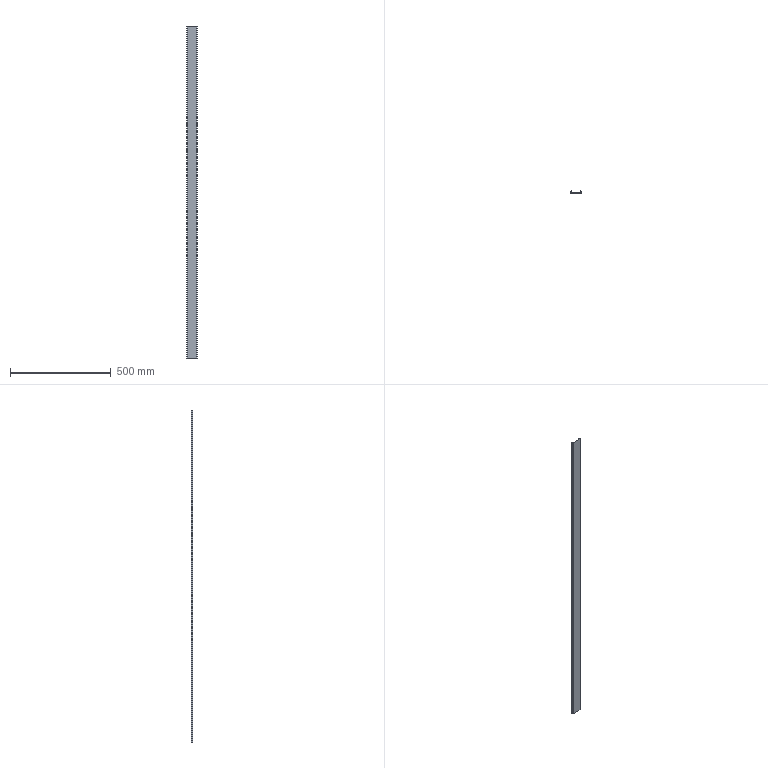Part | STEP file | 46A-00008CC12 | 1 solid | 32 faces | box 50 x 9.195 x 1650 mm | volume 144728 mm3 | plane 16 | cylinder 16 | commonest cylinder face diameters 1 x8 1.2 x6 2 x2
STEP:
#1=CARTESIAN_POINT('',(1.273,9.019,835.));
#2=VERTEX_POINT('',#1);
#3=CARTESIAN_POINT('',(0.4243,9.019,835.));
#4=VERTEX_POINT('',#3);
#5=CARTESIAN_POINT('',(1.273,9.019,835.));
#6=CARTESIAN_POINT('',(1.219,9.073,835.));
#7=CARTESIAN_POINT('',(1.158,9.118,835.));
#8=CARTESIAN_POINT('',(1.089,9.152,835.));
#9=CARTESIAN_POINT('',(0.9442,9.199,835.));
#10=CARTESIAN_POINT('',(0.7916,9.2,835.));
#11=CARTESIAN_POINT('',(0.7159,9.188,835.));
#12=CARTESIAN_POINT('',(0.6071,9.152,835.));
#13=CARTESIAN_POINT('',(0.5104,9.093,835.));
#14=CARTESIAN_POINT('',(0.4796,9.07,835.));
#15=CARTESIAN_POINT('',(0.4509,9.046,835.));
#16=CARTESIAN_POINT('',(0.4243,9.019,835.));
#17=B_SPLINE_CURVE_WITH_KNOTS('',5,(#5,#6,#7,#8,#9,#10,#11,#12,#13,#14,#15,#16),.UNSPECIFIED.,.F.,.U.,(6,3,3,6),(0.,0.5331,1.066,1.332),.UNSPECIFIED.);
#18=EDGE_CURVE('',#2,#4,#17,.T.);
#19=ORIENTED_EDGE('',*,*,#18,.T.);
#20=CARTESIAN_POINT('',(0.2485,8.595,835.));
#21=VERTEX_POINT('',#20);
#22=CARTESIAN_POINT('',(0.4243,9.019,835.));
#23=CARTESIAN_POINT('',(0.3843,8.979,835.));
#24=CARTESIAN_POINT('',(0.349,8.935,835.));
#25=CARTESIAN_POINT('',(0.3192,8.886,835.));
#26=CARTESIAN_POINT('',(0.2795,8.8,835.));
#27=CARTESIAN_POINT('',(0.2574,8.708,835.));
#28=CARTESIAN_POINT('',(0.2515,8.67,835.));
#29=CARTESIAN_POINT('',(0.2485,8.633,835.));
#30=CARTESIAN_POINT('',(0.2485,8.595,835.));
#31=B_SPLINE_CURVE_WITH_KNOTS('',5,(#22,#23,#24,#25,#26,#27,#28,#29,#30),.UNSPECIFIED.,.F.,.U.,(6,3,6),(0.,0.3999,0.6659),.UNSPECIFIED.);
#32=EDGE_CURVE('',#4,#21,#31,.T.);
#33=ORIENTED_EDGE('',*,*,#32,.T.);
#34=CARTESIAN_POINT('',(0.4243,8.171,835.));
#35=VERTEX_POINT('',#34);
#36=CARTESIAN_POINT('',(0.2485,8.595,835.));
#37=CARTESIAN_POINT('',(0.2485,8.538,835.));
#38=CARTESIAN_POINT('',(0.2552,8.482,835.));
#39=CARTESIAN_POINT('',(0.2685,8.426,835.));
#40=CARTESIAN_POINT('',(0.3014,8.337,835.));
#41=CARTESIAN_POINT('',(0.3507,8.257,835.));
#42=CARTESIAN_POINT('',(0.3731,8.226,835.));
#43=CARTESIAN_POINT('',(0.3977,8.197,835.));
#44=CARTESIAN_POINT('',(0.4243,8.171,835.));
#45=B_SPLINE_CURVE_WITH_KNOTS('',5,(#36,#37,#38,#39,#40,#41,#42,#43,#44),.UNSPECIFIED.,.F.,.U.,(6,3,6),(0.,0.3999,0.6659),.UNSPECIFIED.);
#46=EDGE_CURVE('',#21,#35,#45,.T.);
#47=ORIENTED_EDGE('',*,*,#46,.T.);
#48=CARTESIAN_POINT('',(2.898,5.697,835.));
#49=VERTEX_POINT('',#48);
#50=CARTESIAN_POINT('',(1.661,6.934,835.));
#51=DIRECTION('',(0.7071,-0.7071,0.));
#52=VECTOR('',#51,1.);
#53=LINE('',#50,#52);
#54=EDGE_CURVE('',#35,#49,#53,.T.);
#55=ORIENTED_EDGE('',*,*,#54,.T.);
#56=CARTESIAN_POINT('',(0.3706,5.02,835.));
#57=VERTEX_POINT('',#56);
#58=CARTESIAN_POINT('',(1.634,5.359,835.));
#59=DIRECTION('',(-0.9659,-0.2588,0.));
#60=VECTOR('',#59,1.);
#61=LINE('',#58,#60);
#62=EDGE_CURVE('',#49,#57,#61,.T.);
#63=ORIENTED_EDGE('',*,*,#62,.T.);
#64=CARTESIAN_POINT('',(0.,4.537,835.));
#65=VERTEX_POINT('',#64);
#66=CARTESIAN_POINT('',(0.3706,5.02,835.));
#67=CARTESIAN_POINT('',(0.32,5.007,835.));
#68=CARTESIAN_POINT('',(0.2712,4.986,835.));
#69=CARTESIAN_POINT('',(0.2253,4.96,835.));
#70=CARTESIAN_POINT('',(0.1416,4.896,835.));
#71=CARTESIAN_POINT('',(0.07725,4.812,835.));
#72=CARTESIAN_POINT('',(0.05076,4.766,835.));
#73=CARTESIAN_POINT('',(0.02052,4.693,835.));
#74=CARTESIAN_POINT('',(0.005155,4.616,835.));
#75=CARTESIAN_POINT('',(0.001709,4.589,835.));
#76=CARTESIAN_POINT('',(0.,4.563,835.));
#77=CARTESIAN_POINT('',(0.,4.537,835.));
#78=B_SPLINE_CURVE_WITH_KNOTS('',5,(#66,#67,#68,#69,#70,#71,#72,#73,#74,#75,#76,#77),.UNSPECIFIED.,.F.,.U.,(6,3,3,6),(0.,0.3702,0.7405,0.9253),.UNSPECIFIED.);
#79=EDGE_CURVE('',#57,#65,#78,.T.);
#80=ORIENTED_EDGE('',*,*,#79,.T.);
#81=CARTESIAN_POINT('',(0.,1.,835.));
#82=VERTEX_POINT('',#81);
#83=CARTESIAN_POINT('',(0.,2.769,835.));
#84=DIRECTION('',(0.,-1.,0.));
#85=VECTOR('',#84,1.);
#86=LINE('',#83,#85);
#87=EDGE_CURVE('',#65,#82,#86,.T.);
#88=ORIENTED_EDGE('',*,*,#87,.T.);
#89=CARTESIAN_POINT('',(1.,0.,835.));
#90=VERTEX_POINT('',#89);
#91=CARTESIAN_POINT('',(0.,1.,835.));
#92=CARTESIAN_POINT('',(0.,0.902,835.));
#93=CARTESIAN_POINT('',(0.012,0.804,835.));
#94=CARTESIAN_POINT('',(0.036,0.708,835.));
#95=CARTESIAN_POINT('',(0.107,0.5238,835.));
#96=CARTESIAN_POINT('',(0.2204,0.3622,835.));
#97=CARTESIAN_POINT('',(0.2868,0.2888,835.));
#98=CARTESIAN_POINT('',(0.4361,0.1597,835.));
#99=CARTESIAN_POINT('',(0.6122,0.0704,835.));
#100=CARTESIAN_POINT('',(0.7053,0.03682,835.));
#101=CARTESIAN_POINT('',(0.8215,0.01049,835.));
#102=CARTESIAN_POINT('',(0.9393,0.001534,835.));
#103=CARTESIAN_POINT('',(0.9596,0.0005109,835.));
#104=CARTESIAN_POINT('',(0.9798,0.000000001,835.));
#105=CARTESIAN_POINT('',(1.,0.000000001,835.));
#106=B_SPLINE_CURVE_WITH_KNOTS('',5,(#91,#92,#93,#94,#95,#96,#97,#98,#99,#100,#101,#102,#103,#104,#105),.UNSPECIFIED.,.F.,.U.,(6,3,3,3,6),(0.,0.6928,1.386,2.078,2.221),.UNSPECIFIED.);
#107=EDGE_CURVE('',#82,#90,#106,.T.);
#108=ORIENTED_EDGE('',*,*,#107,.T.);
#109=CARTESIAN_POINT('',(49.,0.,835.));
#110=VERTEX_POINT('',#109);
#111=CARTESIAN_POINT('',(25.,0.000000001,835.));
#112=DIRECTION('',(1.,0.,0.));
#113=VECTOR('',#112,1.);
#114=LINE('',#111,#113);
#115=EDGE_CURVE('',#90,#110,#114,.T.);
#116=ORIENTED_EDGE('',*,*,#115,.T.);
#117=CARTESIAN_POINT('',(50.,1.,835.));
#118=VERTEX_POINT('',#117);
#119=CARTESIAN_POINT('',(49.,0.000000001,835.));
#120=CARTESIAN_POINT('',(49.098,0.000000001,835.));
#121=CARTESIAN_POINT('',(49.196,0.012,835.));
#122=CARTESIAN_POINT('',(49.292,0.036,835.));
#123=CARTESIAN_POINT('',(49.476,0.107,835.));
#124=CARTESIAN_POINT('',(49.638,0.2204,835.));
#125=CARTESIAN_POINT('',(49.711,0.2868,835.));
#126=CARTESIAN_POINT('',(49.84,0.4361,835.));
#127=CARTESIAN_POINT('',(49.93,0.6122,835.));
#128=CARTESIAN_POINT('',(49.963,0.7053,835.));
#129=CARTESIAN_POINT('',(49.99,0.8215,835.));
#130=CARTESIAN_POINT('',(49.998,0.9393,835.));
#131=CARTESIAN_POINT('',(49.999,0.9596,835.));
#132=CARTESIAN_POINT('',(50.,0.9798,835.));
#133=CARTESIAN_POINT('',(50.,1.,835.));
#134=B_SPLINE_CURVE_WITH_KNOTS('',5,(#119,#120,#121,#122,#123,#124,#125,#126,#127,#128,#129,#130,#131,#132,#133),.UNSPECIFIED.,.F.,.U.,(6,3,3,3,6),(0.,0.6928,1.386,2.078,2.221),.UNSPECIFIED.);
#135=EDGE_CURVE('',#110,#118,#134,.T.);
#136=ORIENTED_EDGE('',*,*,#135,.T.);
#137=CARTESIAN_POINT('',(50.,4.537,835.));
#138=VERTEX_POINT('',#137);
#139=CARTESIAN_POINT('',(50.,2.769,835.));
#140=DIRECTION('',(0.,1.,0.));
#141=VECTOR('',#140,1.);
#142=LINE('',#139,#141);
#143=EDGE_CURVE('',#118,#138,#142,.T.);
#144=ORIENTED_EDGE('',*,*,#143,.T.);
#145=CARTESIAN_POINT('',(49.629,5.02,835.));
#146=VERTEX_POINT('',#145);
#147=CARTESIAN_POINT('',(50.,4.537,835.));
#148=CARTESIAN_POINT('',(50.,4.589,835.));
#149=CARTESIAN_POINT('',(49.993,4.642,835.));
#150=CARTESIAN_POINT('',(49.979,4.693,835.));
#151=CARTESIAN_POINT('',(49.939,4.791,835.));
#152=CARTESIAN_POINT('',(49.875,4.874,835.));
#153=CARTESIAN_POINT('',(49.837,4.912,835.));
#154=CARTESIAN_POINT('',(49.774,4.96,835.));
#155=CARTESIAN_POINT('',(49.704,4.995,835.));
#156=CARTESIAN_POINT('',(49.679,5.005,835.));
#157=CARTESIAN_POINT('',(49.655,5.013,835.));
#158=CARTESIAN_POINT('',(49.629,5.02,835.));
#159=B_SPLINE_CURVE_WITH_KNOTS('',5,(#147,#148,#149,#150,#151,#152,#153,#154,#155,#156,#157,#158),.UNSPECIFIED.,.F.,.U.,(6,3,3,6),(0.,0.3702,0.7405,0.9253),.UNSPECIFIED.);
#160=EDGE_CURVE('',#138,#146,#159,.T.);
#161=ORIENTED_EDGE('',*,*,#160,.T.);
#162=CARTESIAN_POINT('',(47.102,5.697,835.));
#163=VERTEX_POINT('',#162);
#164=CARTESIAN_POINT('',(48.366,5.359,835.));
#165=DIRECTION('',(-0.9659,0.2588,0.));
#166=VECTOR('',#165,1.);
#167=LINE('',#164,#166);
#168=EDGE_CURVE('',#146,#163,#167,.T.);
#169=ORIENTED_EDGE('',*,*,#168,.T.);
#170=CARTESIAN_POINT('',(49.576,8.171,835.));
#171=VERTEX_POINT('',#170);
#172=CARTESIAN_POINT('',(48.339,6.934,835.));
#173=DIRECTION('',(0.7071,0.7071,0.));
#174=VECTOR('',#173,1.);
#175=LINE('',#172,#174);
#176=EDGE_CURVE('',#163,#171,#175,.T.);
#177=ORIENTED_EDGE('',*,*,#176,.T.);
#178=CARTESIAN_POINT('',(49.751,8.595,835.));
#179=VERTEX_POINT('',#178);
#180=CARTESIAN_POINT('',(49.576,8.171,835.));
#181=CARTESIAN_POINT('',(49.629,8.224,835.));
#182=CARTESIAN_POINT('',(49.674,8.286,835.));
#183=CARTESIAN_POINT('',(49.709,8.354,835.));
#184=CARTESIAN_POINT('',(49.738,8.445,835.));
#185=CARTESIAN_POINT('',(49.749,8.539,835.));
#186=CARTESIAN_POINT('',(49.751,8.557,835.));
#187=CARTESIAN_POINT('',(49.751,8.576,835.));
#188=CARTESIAN_POINT('',(49.751,8.595,835.));
#189=B_SPLINE_CURVE_WITH_KNOTS('',5,(#180,#181,#182,#183,#184,#185,#186,#187,#188),.UNSPECIFIED.,.F.,.U.,(6,3,6),(0.,0.5331,0.6664),.UNSPECIFIED.);
#190=EDGE_CURVE('',#171,#179,#189,.T.);
#191=ORIENTED_EDGE('',*,*,#190,.T.);
#192=CARTESIAN_POINT('',(49.576,9.019,835.));
#193=VERTEX_POINT('',#192);
#194=CARTESIAN_POINT('',(49.751,8.595,835.));
#195=CARTESIAN_POINT('',(49.751,8.652,835.));
#196=CARTESIAN_POINT('',(49.745,8.708,835.));
#197=CARTESIAN_POINT('',(49.731,8.764,835.));
#198=CARTESIAN_POINT('',(49.699,8.853,835.));
#199=CARTESIAN_POINT('',(49.649,8.933,835.));
#200=CARTESIAN_POINT('',(49.627,8.964,835.));
#201=CARTESIAN_POINT('',(49.602,8.993,835.));
#202=CARTESIAN_POINT('',(49.576,9.019,835.));
#203=B_SPLINE_CURVE_WITH_KNOTS('',5,(#194,#195,#196,#197,#198,#199,#200,#201,#202),.UNSPECIFIED.,.F.,.U.,(6,3,6),(0.6664,1.066,1.332),.UNSPECIFIED.);
#204=EDGE_CURVE('',#179,#193,#203,.T.);
#205=ORIENTED_EDGE('',*,*,#204,.T.);
#206=CARTESIAN_POINT('',(48.727,9.019,835.));
#207=VERTEX_POINT('',#206);
#208=CARTESIAN_POINT('',(49.576,9.019,835.));
#209=CARTESIAN_POINT('',(49.522,9.073,835.));
#210=CARTESIAN_POINT('',(49.461,9.118,835.));
#211=CARTESIAN_POINT('',(49.392,9.152,835.));
#212=CARTESIAN_POINT('',(49.247,9.199,835.));
#213=CARTESIAN_POINT('',(49.095,9.2,835.));
#214=CARTESIAN_POINT('',(49.019,9.188,835.));
#215=CARTESIAN_POINT('',(48.91,9.152,835.));
#216=CARTESIAN_POINT('',(48.813,9.093,835.));
#217=CARTESIAN_POINT('',(48.782,9.07,835.));
#218=CARTESIAN_POINT('',(48.754,9.046,835.));
#219=CARTESIAN_POINT('',(48.727,9.019,835.));
#220=B_SPLINE_CURVE_WITH_KNOTS('',5,(#208,#209,#210,#211,#212,#213,#214,#215,#216,#217,#218,#219),.UNSPECIFIED.,.F.,.U.,(6,3,3,6),(0.,0.5331,1.066,1.332),.UNSPECIFIED.);
#221=EDGE_CURVE('',#193,#207,#220,.T.);
#222=ORIENTED_EDGE('',*,*,#221,.T.);
#223=CARTESIAN_POINT('',(45.396,5.688,835.));
#224=VERTEX_POINT('',#223);
#225=CARTESIAN_POINT('',(47.062,7.354,835.));
#226=DIRECTION('',(-0.7071,-0.7071,0.));
#227=VECTOR('',#226,1.);
#228=LINE('',#225,#227);
#229=EDGE_CURVE('',#207,#224,#228,.T.);
#230=ORIENTED_EDGE('',*,*,#229,.T.);
#231=CARTESIAN_POINT('',(45.25,5.335,835.));
#232=VERTEX_POINT('',#231);
#233=CARTESIAN_POINT('',(45.396,5.688,835.));
#234=CARTESIAN_POINT('',(45.363,5.655,835.));
#235=CARTESIAN_POINT('',(45.334,5.618,835.));
#236=CARTESIAN_POINT('',(45.309,5.577,835.));
#237=CARTESIAN_POINT('',(45.276,5.506,835.));
#238=CARTESIAN_POINT('',(45.257,5.429,835.));
#239=CARTESIAN_POINT('',(45.252,5.398,835.));
#240=CARTESIAN_POINT('',(45.25,5.366,835.));
#241=CARTESIAN_POINT('',(45.25,5.335,835.));
#242=B_SPLINE_CURVE_WITH_KNOTS('',5,(#233,#234,#235,#236,#237,#238,#239,#240,#241),.UNSPECIFIED.,.F.,.U.,(6,3,6),(0.,0.3332,0.5549),.UNSPECIFIED.);
#243=EDGE_CURVE('',#224,#232,#242,.T.);
#244=ORIENTED_EDGE('',*,*,#243,.T.);
#245=CARTESIAN_POINT('',(45.621,4.852,835.));
#246=VERTEX_POINT('',#245);
#247=CARTESIAN_POINT('',(45.25,5.335,835.));
#248=CARTESIAN_POINT('',(45.25,5.283,835.));
#249=CARTESIAN_POINT('',(45.257,5.23,835.));
#250=CARTESIAN_POINT('',(45.27,5.179,835.));
#251=CARTESIAN_POINT('',(45.311,5.081,835.));
#252=CARTESIAN_POINT('',(45.375,4.998,835.));
#253=CARTESIAN_POINT('',(45.413,4.96,835.));
#254=CARTESIAN_POINT('',(45.476,4.912,835.));
#255=CARTESIAN_POINT('',(45.546,4.877,835.));
#256=CARTESIAN_POINT('',(45.57,4.867,835.));
#257=CARTESIAN_POINT('',(45.595,4.859,835.));
#258=CARTESIAN_POINT('',(45.621,4.852,835.));
#259=B_SPLINE_CURVE_WITH_KNOTS('',5,(#247,#248,#249,#250,#251,#252,#253,#254,#255,#256,#257,#258),.UNSPECIFIED.,.F.,.U.,(6,3,3,6),(0.,0.3702,0.7405,0.9253),.UNSPECIFIED.);
#260=EDGE_CURVE('',#232,#246,#259,.T.);
#261=ORIENTED_EDGE('',*,*,#260,.T.);
#262=CARTESIAN_POINT('',(48.8,4.,835.));
#263=VERTEX_POINT('',#262);
#264=CARTESIAN_POINT('',(47.21,4.426,835.));
#265=DIRECTION('',(0.9659,-0.2588,0.));
#266=VECTOR('',#265,1.);
#267=LINE('',#264,#266);
#268=EDGE_CURVE('',#246,#263,#267,.T.);
#269=ORIENTED_EDGE('',*,*,#268,.T.);
#270=CARTESIAN_POINT('',(48.8,1.7,835.));
#271=VERTEX_POINT('',#270);
#272=CARTESIAN_POINT('',(48.8,2.85,835.));
#273=DIRECTION('',(0.,-1.,0.));
#274=VECTOR('',#273,1.);
#275=LINE('',#272,#274);
#276=EDGE_CURVE('',#263,#271,#275,.T.);
#277=ORIENTED_EDGE('',*,*,#276,.T.);
#278=CARTESIAN_POINT('',(48.3,1.2,835.));
#279=VERTEX_POINT('',#278);
#280=CARTESIAN_POINT('',(48.3,1.7,835.));
#281=DIRECTION('',(0.,0.,-1.));
#282=AXIS2_PLACEMENT_3D('',#280,#281,$);
#283=CIRCLE('',#282,0.5);
#284=EDGE_CURVE('',#271,#279,#283,.T.);
#285=ORIENTED_EDGE('',*,*,#284,.T.);
#286=CARTESIAN_POINT('',(1.7,1.2,835.));
#287=VERTEX_POINT('',#286);
#288=CARTESIAN_POINT('',(25.,1.2,835.));
#289=DIRECTION('',(-1.,0.,0.));
#290=VECTOR('',#289,1.);
#291=LINE('',#288,#290);
#292=EDGE_CURVE('',#279,#287,#291,.T.);
#293=ORIENTED_EDGE('',*,*,#292,.T.);
#294=CARTESIAN_POINT('',(1.2,1.7,835.));
#295=VERTEX_POINT('',#294);
#296=CARTESIAN_POINT('',(1.7,1.7,835.));
#297=DIRECTION('',(0.,0.,-1.));
#298=AXIS2_PLACEMENT_3D('',#296,#297,$);
#299=CIRCLE('',#298,0.5);
#300=EDGE_CURVE('',#287,#295,#299,.T.);
#301=ORIENTED_EDGE('',*,*,#300,.T.);
#302=CARTESIAN_POINT('',(1.2,4.,835.));
#303=VERTEX_POINT('',#302);
#304=CARTESIAN_POINT('',(1.2,2.85,835.));
#305=DIRECTION('',(0.,1.,0.));
#306=VECTOR('',#305,1.);
#307=LINE('',#304,#306);
#308=EDGE_CURVE('',#295,#303,#307,.T.);
#309=ORIENTED_EDGE('',*,*,#308,.T.);
#310=CARTESIAN_POINT('',(4.379,4.852,835.));
#311=VERTEX_POINT('',#310);
#312=CARTESIAN_POINT('',(2.79,4.426,835.));
#313=DIRECTION('',(0.9659,0.2588,0.));
#314=VECTOR('',#313,1.);
#315=LINE('',#312,#314);
#316=EDGE_CURVE('',#303,#311,#315,.T.);
#317=ORIENTED_EDGE('',*,*,#316,.T.);
#318=CARTESIAN_POINT('',(4.75,5.335,835.));
#319=VERTEX_POINT('',#318);
#320=CARTESIAN_POINT('',(4.379,4.852,835.));
#321=CARTESIAN_POINT('',(4.446,4.87,835.));
#322=CARTESIAN_POINT('',(4.51,4.899,835.));
#323=CARTESIAN_POINT('',(4.568,4.94,835.));
#324=CARTESIAN_POINT('',(4.662,5.034,835.));
#325=CARTESIAN_POINT('',(4.722,5.152,835.));
#326=CARTESIAN_POINT('',(4.741,5.212,835.));
#327=CARTESIAN_POINT('',(4.75,5.273,835.));
#328=CARTESIAN_POINT('',(4.75,5.335,835.));
#329=B_SPLINE_CURVE_WITH_KNOTS('',5,(#320,#321,#322,#323,#324,#325,#326,#327,#328),.UNSPECIFIED.,.F.,.U.,(6,3,6),(0.,0.4899,0.9256),.UNSPECIFIED.);
#330=EDGE_CURVE('',#311,#319,#329,.T.);
#331=ORIENTED_EDGE('',*,*,#330,.T.);
#332=CARTESIAN_POINT('',(4.604,5.688,835.));
#333=VERTEX_POINT('',#332);
#334=CARTESIAN_POINT('',(4.75,5.335,835.));
#335=CARTESIAN_POINT('',(4.75,5.343,835.));
#336=CARTESIAN_POINT('',(4.75,5.35,835.));
#337=CARTESIAN_POINT('',(4.75,5.358,835.));
#338=CARTESIAN_POINT('',(4.745,5.435,835.));
#339=CARTESIAN_POINT('',(4.726,5.51,835.));
#340=CARTESIAN_POINT('',(4.697,5.575,835.));
#341=CARTESIAN_POINT('',(4.657,5.634,835.));
#342=CARTESIAN_POINT('',(4.607,5.685,835.));
#343=CARTESIAN_POINT('',(4.606,5.686,835.));
#344=CARTESIAN_POINT('',(4.605,5.687,835.));
#345=CARTESIAN_POINT('',(4.604,5.688,835.));
#346=B_SPLINE_CURVE_WITH_KNOTS('',5,(#334,#335,#336,#337,#338,#339,#340,#341,#342,#343,#344,#345),.UNSPECIFIED.,.F.,.U.,(6,3,3,6),(0.9256,0.9798,1.47,1.481),.UNSPECIFIED.);
#347=EDGE_CURVE('',#319,#333,#346,.T.);
#348=ORIENTED_EDGE('',*,*,#347,.T.);
#349=CARTESIAN_POINT('',(2.938,7.354,835.));
#350=DIRECTION('',(-0.7071,0.7071,0.));
#351=VECTOR('',#350,1.);
#352=LINE('',#349,#351);
#353=EDGE_CURVE('',#333,#2,#352,.T.);
#354=ORIENTED_EDGE('',*,*,#353,.T.);
#355=EDGE_LOOP('',(#19,#33,#47,#55,#63,#80,#88,#108,#116,#136,#144,#161,#169,#177,#191,#205,#222,#230,#244,#261,#269,#277,#285,#293,#301,#309,#317,#331,#348,#354));
#356=FACE_OUTER_BOUND('',#355,.T.);
#357=CARTESIAN_POINT('',(0.,1.2,835.));
#358=DIRECTION('',(0.,0.,-1.));
#359=DIRECTION('',(-1.,0.,0.));
#360=AXIS2_PLACEMENT_3D('',#357,#358,#359);
#361=PLANE('',#360);
#362=ADVANCED_FACE('',(#356),#361,.F.);
#363=CARTESIAN_POINT('',(1.273,9.019,-815.));
#364=VERTEX_POINT('',#363);
#365=CARTESIAN_POINT('',(4.604,5.688,-815.));
#366=VERTEX_POINT('',#365);
#367=CARTESIAN_POINT('',(2.938,7.354,-815.));
#368=DIRECTION('',(0.7071,-0.7071,0.));
#369=VECTOR('',#368,1.);
#370=LINE('',#367,#369);
#371=EDGE_CURVE('',#364,#366,#370,.T.);
#372=ORIENTED_EDGE('',*,*,#371,.F.);
#373=CARTESIAN_POINT('',(1.273,9.019,10.));
#374=DIRECTION('',(0.,0.,1.));
#375=VECTOR('',#374,1.);
#376=LINE('',#373,#375);
#377=EDGE_CURVE('',#364,#2,#376,.T.);
#378=ORIENTED_EDGE('',*,*,#377,.T.);
#379=ORIENTED_EDGE('',*,*,#353,.F.);
#380=CARTESIAN_POINT('',(4.604,5.688,10.));
#381=DIRECTION('',(0.,0.,-1.));
#382=VECTOR('',#381,1.);
#383=LINE('',#380,#382);
#384=EDGE_CURVE('',#333,#366,#383,.T.);
#385=ORIENTED_EDGE('',*,*,#384,.T.);
#386=EDGE_LOOP('',(#372,#378,#379,#385));
#387=FACE_OUTER_BOUND('',#386,.T.);
#388=CARTESIAN_POINT('',(5.216,5.076,835.));
#389=DIRECTION('',(-0.7071,-0.7071,0.));
#390=DIRECTION('',(0.7071,-0.7071,0.));
#391=AXIS2_PLACEMENT_3D('',#388,#389,#390);
#392=PLANE('',#391);
#393=ADVANCED_FACE('',(#387),#392,.F.);
#394=ORIENTED_EDGE('',*,*,#384,.F.);
#395=ORIENTED_EDGE('',*,*,#347,.F.);
#396=CARTESIAN_POINT('',(4.75,5.335,-815.));
#397=VERTEX_POINT('',#396);
#398=CARTESIAN_POINT('',(4.75,5.335,835.));
#399=DIRECTION('',(0.,0.,-1.));
#400=VECTOR('',#399,1.);
#401=LINE('',#398,#400);
#402=EDGE_CURVE('',#319,#397,#401,.T.);
#403=ORIENTED_EDGE('',*,*,#402,.T.);
#404=CARTESIAN_POINT('',(4.25,5.335,-815.));
#405=DIRECTION('',(0.,0.,-1.));
#406=AXIS2_PLACEMENT_3D('',#404,#405,$);
#407=CIRCLE('',#406,0.5);
#408=EDGE_CURVE('',#366,#397,#407,.T.);
#409=ORIENTED_EDGE('',*,*,#408,.F.);
#410=EDGE_LOOP('',(#394,#395,#403,#409));
#411=FACE_OUTER_BOUND('',#410,.T.);
#412=CARTESIAN_POINT('',(4.25,5.335,835.));
#413=DIRECTION('',(0.,0.,-1.));
#414=DIRECTION('',(-1.,0.,0.));
#415=AXIS2_PLACEMENT_3D('',#412,#413,#414);
#416=CYLINDRICAL_SURFACE('',#415,0.5);
#417=ADVANCED_FACE('',(#411),#416,.T.);
#418=ORIENTED_EDGE('',*,*,#402,.F.);
#419=ORIENTED_EDGE('',*,*,#330,.F.);
#420=CARTESIAN_POINT('',(4.379,4.852,-815.));
#421=VERTEX_POINT('',#420);
#422=CARTESIAN_POINT('',(4.379,4.852,835.));
#423=DIRECTION('',(0.,0.,-1.));
#424=VECTOR('',#423,1.);
#425=LINE('',#422,#424);
#426=EDGE_CURVE('',#421,#311,#425,.F.);
#427=ORIENTED_EDGE('',*,*,#426,.F.);
#428=CARTESIAN_POINT('',(4.25,5.335,-815.));
#429=DIRECTION('',(0.,0.,-1.));
#430=AXIS2_PLACEMENT_3D('',#428,#429,$);
#431=CIRCLE('',#430,0.5);
#432=EDGE_CURVE('',#397,#421,#431,.T.);
#433=ORIENTED_EDGE('',*,*,#432,.F.);
#434=EDGE_LOOP('',(#418,#419,#427,#433));
#435=FACE_OUTER_BOUND('',#434,.T.);
#436=CARTESIAN_POINT('',(4.25,5.335,835.));
#437=DIRECTION('',(0.,0.,-1.));
#438=DIRECTION('',(1.,0.,0.));
#439=AXIS2_PLACEMENT_3D('',#436,#437,#438);
#440=CYLINDRICAL_SURFACE('',#439,0.5);
#441=ADVANCED_FACE('',(#435),#440,.T.);
#442=ORIENTED_EDGE('',*,*,#316,.F.);
#443=CARTESIAN_POINT('',(1.2,4.,-815.));
#444=VERTEX_POINT('',#443);
#445=CARTESIAN_POINT('',(1.2,4.,10.));
#446=DIRECTION('',(0.,0.,1.));
#447=VECTOR('',#446,1.);
#448=LINE('',#445,#447);
#449=EDGE_CURVE('',#444,#303,#448,.T.);
#450=ORIENTED_EDGE('',*,*,#449,.F.);
#451=CARTESIAN_POINT('',(2.79,4.426,-815.));
#452=DIRECTION('',(-0.9659,-0.2588,0.));
#453=VECTOR('',#452,1.);
#454=LINE('',#451,#453);
#455=EDGE_CURVE('',#421,#444,#454,.T.);
#456=ORIENTED_EDGE('',*,*,#455,.F.);
#457=ORIENTED_EDGE('',*,*,#426,.T.);
#458=EDGE_LOOP('',(#442,#450,#456,#457));
#459=FACE_OUTER_BOUND('',#458,.T.);
#460=CARTESIAN_POINT('',(1.2,4.,835.));
#461=DIRECTION('',(-0.2588,0.9659,0.));
#462=DIRECTION('',(-0.9659,-0.2588,0.));
#463=AXIS2_PLACEMENT_3D('',#460,#461,#462);
#464=PLANE('',#463);
#465=ADVANCED_FACE('',(#459),#464,.F.);
#466=ORIENTED_EDGE('',*,*,#308,.F.);
#467=CARTESIAN_POINT('',(1.2,1.7,-815.));
#468=VERTEX_POINT('',#467);
#469=CARTESIAN_POINT('',(1.2,1.7,10.));
#470=DIRECTION('',(0.,0.,-1.));
#471=VECTOR('',#470,1.);
#472=LINE('',#469,#471);
#473=EDGE_CURVE('',#295,#468,#472,.T.);
#474=ORIENTED_EDGE('',*,*,#473,.T.);
#475=CARTESIAN_POINT('',(1.2,2.85,-815.));
#476=DIRECTION('',(0.,-1.,0.));
#477=VECTOR('',#476,1.);
#478=LINE('',#475,#477);
#479=EDGE_CURVE('',#444,#468,#478,.T.);
#480=ORIENTED_EDGE('',*,*,#479,.F.);
#481=ORIENTED_EDGE('',*,*,#449,.T.);
#482=EDGE_LOOP('',(#466,#474,#480,#481));
#483=FACE_OUTER_BOUND('',#482,.T.);
#484=CARTESIAN_POINT('',(1.2,1.2,835.));
#485=DIRECTION('',(-1.,0.,0.));
#486=DIRECTION('',(0.,0.,1.));
#487=AXIS2_PLACEMENT_3D('',#484,#485,#486);
#488=PLANE('',#487);
#489=ADVANCED_FACE('',(#483),#488,.F.);
#490=ORIENTED_EDGE('',*,*,#300,.F.);
#491=CARTESIAN_POINT('',(1.7,1.2,-815.));
#492=VERTEX_POINT('',#491);
#493=CARTESIAN_POINT('',(1.7,1.2,835.));
#494=DIRECTION('',(0.,0.,1.));
#495=VECTOR('',#494,1.);
#496=LINE('',#493,#495);
#497=EDGE_CURVE('',#492,#287,#496,.T.);
#498=ORIENTED_EDGE('',*,*,#497,.F.);
#499=CARTESIAN_POINT('',(1.7,1.7,-815.));
#500=DIRECTION('',(0.,0.,1.));
#501=AXIS2_PLACEMENT_3D('',#499,#500,$);
#502=CIRCLE('',#501,0.5);
#503=EDGE_CURVE('',#468,#492,#502,.T.);
#504=ORIENTED_EDGE('',*,*,#503,.F.);
#505=ORIENTED_EDGE('',*,*,#473,.F.);
#506=EDGE_LOOP('',(#490,#498,#504,#505));
#507=FACE_OUTER_BOUND('',#506,.T.);
#508=CARTESIAN_POINT('',(1.7,1.7,835.));
#509=DIRECTION('',(0.,0.,1.));
#510=DIRECTION('',(-1.,0.,0.));
#511=AXIS2_PLACEMENT_3D('',#508,#509,#510);
#512=CYLINDRICAL_SURFACE('',#511,0.5);
#513=ADVANCED_FACE('',(#507),#512,.F.);
#514=ORIENTED_EDGE('',*,*,#292,.F.);
#515=CARTESIAN_POINT('',(48.3,1.2,-815.));
#516=VERTEX_POINT('',#515);
#517=CARTESIAN_POINT('',(48.3,1.2,10.));
#518=DIRECTION('',(0.,0.,-1.));
#519=VECTOR('',#518,1.);
#520=LINE('',#517,#519);
#521=EDGE_CURVE('',#279,#516,#520,.T.);
#522=ORIENTED_EDGE('',*,*,#521,.T.);
#523=CARTESIAN_POINT('',(25.,1.2,-815.));
#524=DIRECTION('',(1.,0.,0.));
#525=VECTOR('',#524,1.);
#526=LINE('',#523,#525);
#527=EDGE_CURVE('',#492,#516,#526,.T.);
#528=ORIENTED_EDGE('',*,*,#527,.F.);
#529=ORIENTED_EDGE('',*,*,#497,.T.);
#530=EDGE_LOOP('',(#514,#522,#528,#529));
#531=FACE_OUTER_BOUND('',#530,.T.);
#532=CARTESIAN_POINT('',(1.2,1.2,835.));
#533=DIRECTION('',(0.,-1.,0.));
#534=DIRECTION('',(0.,0.,-1.));
#535=AXIS2_PLACEMENT_3D('',#532,#533,#534);
#536=PLANE('',#535);
#537=ADVANCED_FACE('',(#531),#536,.F.);
#538=ORIENTED_EDGE('',*,*,#284,.F.);
#539=CARTESIAN_POINT('',(48.8,1.7,-815.));
#540=VERTEX_POINT('',#539);
#541=CARTESIAN_POINT('',(48.8,1.7,835.));
#542=DIRECTION('',(0.,0.,1.));
#543=VECTOR('',#542,1.);
#544=LINE('',#541,#543);
#545=EDGE_CURVE('',#540,#271,#544,.T.);
#546=ORIENTED_EDGE('',*,*,#545,.F.);
#547=CARTESIAN_POINT('',(48.3,1.7,-815.));
#548=DIRECTION('',(0.,0.,1.));
#549=AXIS2_PLACEMENT_3D('',#547,#548,$);
#550=CIRCLE('',#549,0.5);
#551=EDGE_CURVE('',#516,#540,#550,.T.);
#552=ORIENTED_EDGE('',*,*,#551,.F.);
#553=ORIENTED_EDGE('',*,*,#521,.F.);
#554=EDGE_LOOP('',(#538,#546,#552,#553));
#555=FACE_OUTER_BOUND('',#554,.T.);
#556=CARTESIAN_POINT('',(48.3,1.7,835.));
#557=DIRECTION('',(0.,0.,1.));
#558=DIRECTION('',(-1.,0.,0.));
#559=AXIS2_PLACEMENT_3D('',#556,#557,#558);
#560=CYLINDRICAL_SURFACE('',#559,0.5);
#561=ADVANCED_FACE('',(#555),#560,.F.);
#562=ORIENTED_EDGE('',*,*,#276,.F.);
#563=CARTESIAN_POINT('',(48.8,4.,-815.));
#564=VERTEX_POINT('',#563);
#565=CARTESIAN_POINT('',(48.8,4.,10.));
#566=DIRECTION('',(0.,0.,1.));
#567=VECTOR('',#566,1.);
#568=LINE('',#565,#567);
#569=EDGE_CURVE('',#564,#263,#568,.T.);
#570=ORIENTED_EDGE('',*,*,#569,.F.);
#571=CARTESIAN_POINT('',(48.8,2.85,-815.));
#572=DIRECTION('',(0.,1.,0.));
#573=VECTOR('',#572,1.);
#574=LINE('',#571,#573);
#575=EDGE_CURVE('',#540,#564,#574,.T.);
#576=ORIENTED_EDGE('',*,*,#575,.F.);
#577=ORIENTED_EDGE('',*,*,#545,.T.);
#578=EDGE_LOOP('',(#562,#570,#576,#577));
#579=FACE_OUTER_BOUND('',#578,.T.);
#580=CARTESIAN_POINT('',(48.8,1.2,835.));
#581=DIRECTION('',(1.,0.,0.));
#582=DIRECTION('',(0.,1.,0.));
#583=AXIS2_PLACEMENT_3D('',#580,#581,#582);
#584=PLANE('',#583);
#585=ADVANCED_FACE('',(#579),#584,.F.);
#586=ORIENTED_EDGE('',*,*,#268,.F.);
#587=CARTESIAN_POINT('',(45.621,4.852,-815.));
#588=VERTEX_POINT('',#587);
#589=CARTESIAN_POINT('',(45.621,4.852,10.));
#590=DIRECTION('',(0.,0.,-1.));
#591=VECTOR('',#590,1.);
#592=LINE('',#589,#591);
#593=EDGE_CURVE('',#246,#588,#592,.T.);
#594=ORIENTED_EDGE('',*,*,#593,.T.);
#595=CARTESIAN_POINT('',(47.21,4.426,-815.));
#596=DIRECTION('',(-0.9659,0.2588,0.));
#597=VECTOR('',#596,1.);
#598=LINE('',#595,#597);
#599=EDGE_CURVE('',#564,#588,#598,.T.);
#600=ORIENTED_EDGE('',*,*,#599,.F.);
#601=ORIENTED_EDGE('',*,*,#569,.T.);
#602=EDGE_LOOP('',(#586,#594,#600,#601));
#603=FACE_OUTER_BOUND('',#602,.T.);
#604=CARTESIAN_POINT('',(48.8,4.,835.));
#605=DIRECTION('',(0.2588,0.9659,0.));
#606=DIRECTION('',(-0.9659,0.2588,0.));
#607=AXIS2_PLACEMENT_3D('',#604,#605,#606);
#608=PLANE('',#607);
#609=ADVANCED_FACE('',(#603),#608,.F.);
#610=ORIENTED_EDGE('',*,*,#593,.F.);
#611=ORIENTED_EDGE('',*,*,#260,.F.);
#612=CARTESIAN_POINT('',(45.25,5.335,-815.));
#613=VERTEX_POINT('',#612);
#614=CARTESIAN_POINT('',(45.25,5.335,835.));
#615=DIRECTION('',(0.,0.,-1.));
#616=VECTOR('',#615,1.);
#617=LINE('',#614,#616);
#618=EDGE_CURVE('',#232,#613,#617,.T.);
#619=ORIENTED_EDGE('',*,*,#618,.T.);
#620=CARTESIAN_POINT('',(45.75,5.335,-815.));
#621=DIRECTION('',(0.,0.,-1.));
#622=AXIS2_PLACEMENT_3D('',#620,#621,$);
#623=CIRCLE('',#622,0.5);
#624=EDGE_CURVE('',#588,#613,#623,.T.);
#625=ORIENTED_EDGE('',*,*,#624,.F.);
#626=EDGE_LOOP('',(#610,#611,#619,#625));
#627=FACE_OUTER_BOUND('',#626,.T.);
#628=CARTESIAN_POINT('',(45.75,5.335,835.));
#629=DIRECTION('',(0.,0.,-1.));
#630=DIRECTION('',(1.,0.,0.));
#631=AXIS2_PLACEMENT_3D('',#628,#629,#630);
#632=CYLINDRICAL_SURFACE('',#631,0.5);
#633=ADVANCED_FACE('',(#627),#632,.T.);
#634=ORIENTED_EDGE('',*,*,#618,.F.);
#635=ORIENTED_EDGE('',*,*,#243,.F.);
#636=CARTESIAN_POINT('',(45.396,5.688,-815.));
#637=VERTEX_POINT('',#636);
#638=CARTESIAN_POINT('',(45.396,5.688,835.));
#639=DIRECTION('',(0.,0.,-1.));
#640=VECTOR('',#639,1.);
#641=LINE('',#638,#640);
#642=EDGE_CURVE('',#637,#224,#641,.F.);
#643=ORIENTED_EDGE('',*,*,#642,.F.);
#644=CARTESIAN_POINT('',(45.75,5.335,-815.));
#645=DIRECTION('',(0.,0.,-1.));
#646=AXIS2_PLACEMENT_3D('',#644,#645,$);
#647=CIRCLE('',#646,0.5);
#648=EDGE_CURVE('',#613,#637,#647,.T.);
#649=ORIENTED_EDGE('',*,*,#648,.F.);
#650=EDGE_LOOP('',(#634,#635,#643,#649));
#651=FACE_OUTER_BOUND('',#650,.T.);
#652=CARTESIAN_POINT('',(45.75,5.335,835.));
#653=DIRECTION('',(0.,0.,-1.));
#654=DIRECTION('',(-1.,0.,0.));
#655=AXIS2_PLACEMENT_3D('',#652,#653,#654);
#656=CYLINDRICAL_SURFACE('',#655,0.5);
#657=ADVANCED_FACE('',(#651),#656,.T.);
#658=ORIENTED_EDGE('',*,*,#229,.F.);
#659=CARTESIAN_POINT('',(48.727,9.019,-815.));
#660=VERTEX_POINT('',#659);
#661=CARTESIAN_POINT('',(48.727,9.019,10.));
#662=DIRECTION('',(0.,0.,-1.));
#663=VECTOR('',#662,1.);
#664=LINE('',#661,#663);
#665=EDGE_CURVE('',#207,#660,#664,.T.);
#666=ORIENTED_EDGE('',*,*,#665,.T.);
#667=CARTESIAN_POINT('',(47.062,7.354,-815.));
#668=DIRECTION('',(0.7071,0.7071,0.));
#669=VECTOR('',#668,1.);
#670=LINE('',#667,#669);
#671=EDGE_CURVE('',#637,#660,#670,.T.);
#672=ORIENTED_EDGE('',*,*,#671,.F.);
#673=ORIENTED_EDGE('',*,*,#642,.T.);
#674=EDGE_LOOP('',(#658,#666,#672,#673));
#675=FACE_OUTER_BOUND('',#674,.T.);
#676=CARTESIAN_POINT('',(44.784,5.076,835.));
#677=DIRECTION('',(0.7071,-0.7071,0.));
#678=DIRECTION('',(0.7071,0.7071,0.));
#679=AXIS2_PLACEMENT_3D('',#676,#677,#678);
#680=PLANE('',#679);
#681=ADVANCED_FACE('',(#675),#680,.F.);
#682=ORIENTED_EDGE('',*,*,#665,.F.);
#683=ORIENTED_EDGE('',*,*,#221,.F.);
#684=CARTESIAN_POINT('',(49.576,9.019,-815.));
#685=VERTEX_POINT('',#684);
#686=CARTESIAN_POINT('',(49.576,9.019,835.));
#687=DIRECTION('',(0.,0.,-1.));
#688=VECTOR('',#687,1.);
#689=LINE('',#686,#688);
#690=EDGE_CURVE('',#193,#685,#689,.T.);
#691=ORIENTED_EDGE('',*,*,#690,.T.);
#692=CARTESIAN_POINT('',(49.151,8.595,-815.));
#693=DIRECTION('',(0.,0.,-1.));
#694=AXIS2_PLACEMENT_3D('',#692,#693,$);
#695=CIRCLE('',#694,0.6);
#696=EDGE_CURVE('',#660,#685,#695,.T.);
#697=ORIENTED_EDGE('',*,*,#696,.F.);
#698=EDGE_LOOP('',(#682,#683,#691,#697));
#699=FACE_OUTER_BOUND('',#698,.T.);
#700=CARTESIAN_POINT('',(49.151,8.595,835.));
#701=DIRECTION('',(0.,0.,-1.));
#702=DIRECTION('',(-1.,0.,0.));
#703=AXIS2_PLACEMENT_3D('',#700,#701,#702);
#704=CYLINDRICAL_SURFACE('',#703,0.6);
#705=ADVANCED_FACE('',(#699),#704,.T.);
#706=ORIENTED_EDGE('',*,*,#690,.F.);
#707=ORIENTED_EDGE('',*,*,#204,.F.);
#708=CARTESIAN_POINT('',(49.751,8.595,-815.));
#709=VERTEX_POINT('',#708);
#710=CARTESIAN_POINT('',(49.751,8.595,835.));
#711=DIRECTION('',(0.,0.,-1.));
#712=VECTOR('',#711,1.);
#713=LINE('',#710,#712);
#714=EDGE_CURVE('',#179,#709,#713,.T.);
#715=ORIENTED_EDGE('',*,*,#714,.T.);
#716=CARTESIAN_POINT('',(49.151,8.595,-815.));
#717=DIRECTION('',(0.,0.,-1.));
#718=AXIS2_PLACEMENT_3D('',#716,#717,$);
#719=CIRCLE('',#718,0.6);
#720=EDGE_CURVE('',#685,#709,#719,.T.);
#721=ORIENTED_EDGE('',*,*,#720,.F.);
#722=EDGE_LOOP('',(#706,#707,#715,#721));
#723=FACE_OUTER_BOUND('',#722,.T.);
#724=CARTESIAN_POINT('',(49.151,8.595,835.));
#725=DIRECTION('',(0.,0.,-1.));
#726=DIRECTION('',(-1.,0.,0.));
#727=AXIS2_PLACEMENT_3D('',#724,#725,#726);
#728=CYLINDRICAL_SURFACE('',#727,0.6);
#729=ADVANCED_FACE('',(#723),#728,.T.);
#730=ORIENTED_EDGE('',*,*,#714,.F.);
#731=ORIENTED_EDGE('',*,*,#190,.F.);
#732=CARTESIAN_POINT('',(49.576,8.171,-815.));
#733=VERTEX_POINT('',#732);
#734=CARTESIAN_POINT('',(49.576,8.171,835.));
#735=DIRECTION('',(0.,0.,-1.));
#736=VECTOR('',#735,1.);
#737=LINE('',#734,#736);
#738=EDGE_CURVE('',#733,#171,#737,.F.);
#739=ORIENTED_EDGE('',*,*,#738,.F.);
#740=CARTESIAN_POINT('',(49.151,8.595,-815.));
#741=DIRECTION('',(0.,0.,-1.));
#742=AXIS2_PLACEMENT_3D('',#740,#741,$);
#743=CIRCLE('',#742,0.6);
#744=EDGE_CURVE('',#709,#733,#743,.T.);
#745=ORIENTED_EDGE('',*,*,#744,.F.);
#746=EDGE_LOOP('',(#730,#731,#739,#745));
#747=FACE_OUTER_BOUND('',#746,.T.);
#748=CARTESIAN_POINT('',(49.151,8.595,835.));
#749=DIRECTION('',(0.,0.,-1.));
#750=DIRECTION('',(1.,0.,0.));
#751=AXIS2_PLACEMENT_3D('',#748,#749,#750);
#752=CYLINDRICAL_SURFACE('',#751,0.6);
#753=ADVANCED_FACE('',(#747),#752,.T.);
#754=ORIENTED_EDGE('',*,*,#176,.F.);
#755=CARTESIAN_POINT('',(47.102,5.697,-815.));
#756=VERTEX_POINT('',#755);
#757=CARTESIAN_POINT('',(47.102,5.697,10.));
#758=DIRECTION('',(0.,0.,1.));
#759=VECTOR('',#758,1.);
#760=LINE('',#757,#759);
#761=EDGE_CURVE('',#756,#163,#760,.T.);
#762=ORIENTED_EDGE('',*,*,#761,.F.);
#763=CARTESIAN_POINT('',(48.339,6.934,-815.));
#764=DIRECTION('',(-0.7071,-0.7071,0.));
#765=VECTOR('',#764,1.);
#766=LINE('',#763,#765);
#767=EDGE_CURVE('',#733,#756,#766,.T.);
#768=ORIENTED_EDGE('',*,*,#767,.F.);
#769=ORIENTED_EDGE('',*,*,#738,.T.);
#770=EDGE_LOOP('',(#754,#762,#768,#769));
#771=FACE_OUTER_BOUND('',#770,.T.);
#772=CARTESIAN_POINT('',(47.102,5.697,835.));
#773=DIRECTION('',(-0.7071,0.7071,0.));
#774=DIRECTION('',(-0.7071,-0.7071,0.));
#775=AXIS2_PLACEMENT_3D('',#772,#773,#774);
#776=PLANE('',#775);
#777=ADVANCED_FACE('',(#771),#776,.F.);
#778=ORIENTED_EDGE('',*,*,#168,.F.);
#779=CARTESIAN_POINT('',(49.629,5.02,-815.));
#780=VERTEX_POINT('',#779);
#781=CARTESIAN_POINT('',(49.629,5.02,10.));
#782=DIRECTION('',(0.,0.,-1.));
#783=VECTOR('',#782,1.);
#784=LINE('',#781,#783);
#785=EDGE_CURVE('',#146,#780,#784,.T.);
#786=ORIENTED_EDGE('',*,*,#785,.T.);
#787=CARTESIAN_POINT('',(48.366,5.359,-815.));
#788=DIRECTION('',(0.9659,-0.2588,0.));
#789=VECTOR('',#788,1.);
#790=LINE('',#787,#789);
#791=EDGE_CURVE('',#756,#780,#790,.T.);
#792=ORIENTED_EDGE('',*,*,#791,.F.);
#793=ORIENTED_EDGE('',*,*,#761,.T.);
#794=EDGE_LOOP('',(#778,#786,#792,#793));
#795=FACE_OUTER_BOUND('',#794,.T.);
#796=CARTESIAN_POINT('',(50.,4.921,835.));
#797=DIRECTION('',(-0.2588,-0.9659,0.));
#798=DIRECTION('',(0.9659,-0.2588,0.));
#799=AXIS2_PLACEMENT_3D('',#796,#797,#798);
#800=PLANE('',#799);
#801=ADVANCED_FACE('',(#795),#800,.F.);
#802=ORIENTED_EDGE('',*,*,#785,.F.);
#803=ORIENTED_EDGE('',*,*,#160,.F.);
#804=CARTESIAN_POINT('',(50.,4.537,-815.));
#805=VERTEX_POINT('',#804);
#806=CARTESIAN_POINT('',(50.,4.537,835.));
#807=DIRECTION('',(0.,0.,-1.));
#808=VECTOR('',#807,1.);
#809=LINE('',#806,#808);
#810=EDGE_CURVE('',#805,#138,#809,.F.);
#811=ORIENTED_EDGE('',*,*,#810,.F.);
#812=CARTESIAN_POINT('',(49.5,4.537,-815.));
#813=DIRECTION('',(0.,0.,-1.));
#814=AXIS2_PLACEMENT_3D('',#812,#813,$);
#815=CIRCLE('',#814,0.5);
#816=EDGE_CURVE('',#780,#805,#815,.T.);
#817=ORIENTED_EDGE('',*,*,#816,.F.);
#818=EDGE_LOOP('',(#802,#803,#811,#817));
#819=FACE_OUTER_BOUND('',#818,.T.);
#820=CARTESIAN_POINT('',(49.5,4.537,835.));
#821=DIRECTION('',(0.,0.,-1.));
#822=DIRECTION('',(-1.,0.,0.));
#823=AXIS2_PLACEMENT_3D('',#820,#821,#822);
#824=CYLINDRICAL_SURFACE('',#823,0.5);
#825=ADVANCED_FACE('',(#819),#824,.T.);
#826=ORIENTED_EDGE('',*,*,#143,.F.);
#827=CARTESIAN_POINT('',(50.,1.,-815.));
#828=VERTEX_POINT('',#827);
#829=CARTESIAN_POINT('',(50.,1.,10.));
#830=DIRECTION('',(0.,0.,-1.));
#831=VECTOR('',#830,1.);
#832=LINE('',#829,#831);
#833=EDGE_CURVE('',#118,#828,#832,.T.);
#834=ORIENTED_EDGE('',*,*,#833,.T.);
#835=CARTESIAN_POINT('',(50.,2.769,-815.));
#836=DIRECTION('',(0.,-1.,0.));
#837=VECTOR('',#836,1.);
#838=LINE('',#835,#837);
#839=EDGE_CURVE('',#805,#828,#838,.T.);
#840=ORIENTED_EDGE('',*,*,#839,.F.);
#841=ORIENTED_EDGE('',*,*,#810,.T.);
#842=EDGE_LOOP('',(#826,#834,#840,#841));
#843=FACE_OUTER_BOUND('',#842,.T.);
#844=CARTESIAN_POINT('',(50.,0.,835.));
#845=DIRECTION('',(-1.,0.,0.));
#846=DIRECTION('',(0.,-1.,0.));
#847=AXIS2_PLACEMENT_3D('',#844,#845,#846);
#848=PLANE('',#847);
#849=ADVANCED_FACE('',(#843),#848,.F.);
#850=ORIENTED_EDGE('',*,*,#833,.F.);
#851=ORIENTED_EDGE('',*,*,#135,.F.);
#852=CARTESIAN_POINT('',(49.,0.,-815.));
#853=VERTEX_POINT('',#852);
#854=CARTESIAN_POINT('',(49.,0.,835.));
#855=DIRECTION('',(0.,0.,-1.));
#856=VECTOR('',#855,1.);
#857=LINE('',#854,#856);
#858=EDGE_CURVE('',#853,#110,#857,.F.);
#859=ORIENTED_EDGE('',*,*,#858,.F.);
#860=CARTESIAN_POINT('',(49.,1.,-815.));
#861=DIRECTION('',(0.,0.,-1.));
#862=AXIS2_PLACEMENT_3D('',#860,#861,$);
#863=CIRCLE('',#862,1.);
#864=EDGE_CURVE('',#828,#853,#863,.T.);
#865=ORIENTED_EDGE('',*,*,#864,.F.);
#866=EDGE_LOOP('',(#850,#851,#859,#865));
#867=FACE_OUTER_BOUND('',#866,.T.);
#868=CARTESIAN_POINT('',(49.,1.,835.));
#869=DIRECTION('',(0.,0.,-1.));
#870=DIRECTION('',(1.,0.,0.));
#871=AXIS2_PLACEMENT_3D('',#868,#869,#870);
#872=CYLINDRICAL_SURFACE('',#871,1.);
#873=ADVANCED_FACE('',(#867),#872,.T.);
#874=ORIENTED_EDGE('',*,*,#115,.F.);
#875=CARTESIAN_POINT('',(1.,0.,-815.));
#876=VERTEX_POINT('',#875);
#877=CARTESIAN_POINT('',(1.,0.,10.));
#878=DIRECTION('',(0.,0.,-1.));
#879=VECTOR('',#878,1.);
#880=LINE('',#877,#879);
#881=EDGE_CURVE('',#90,#876,#880,.T.);
#882=ORIENTED_EDGE('',*,*,#881,.T.);
#883=CARTESIAN_POINT('',(25.,0.,-815.));
#884=DIRECTION('',(-1.,0.,0.));
#885=VECTOR('',#884,1.);
#886=LINE('',#883,#885);
#887=EDGE_CURVE('',#853,#876,#886,.T.);
#888=ORIENTED_EDGE('',*,*,#887,.F.);
#889=ORIENTED_EDGE('',*,*,#858,.T.);
#890=EDGE_LOOP('',(#874,#882,#888,#889));
#891=FACE_OUTER_BOUND('',#890,.T.);
#892=CARTESIAN_POINT('',(0.,0.,835.));
#893=DIRECTION('',(0.,1.,0.));
#894=DIRECTION('',(-1.,0.,0.));
#895=AXIS2_PLACEMENT_3D('',#892,#893,#894);
#896=PLANE('',#895);
#897=ADVANCED_FACE('',(#891),#896,.F.);
#898=ORIENTED_EDGE('',*,*,#881,.F.);
#899=ORIENTED_EDGE('',*,*,#107,.F.);
#900=CARTESIAN_POINT('',(0.,1.,-815.));
#901=VERTEX_POINT('',#900);
#902=CARTESIAN_POINT('',(0.,1.,835.));
#903=DIRECTION('',(0.,0.,-1.));
#904=VECTOR('',#903,1.);
#905=LINE('',#902,#904);
#906=EDGE_CURVE('',#901,#82,#905,.F.);
#907=ORIENTED_EDGE('',*,*,#906,.F.);
#908=CARTESIAN_POINT('',(1.,1.,-815.));
#909=DIRECTION('',(0.,0.,-1.));
#910=AXIS2_PLACEMENT_3D('',#908,#909,$);
#911=CIRCLE('',#910,1.);
#912=EDGE_CURVE('',#876,#901,#911,.T.);
#913=ORIENTED_EDGE('',*,*,#912,.F.);
#914=EDGE_LOOP('',(#898,#899,#907,#913));
#915=FACE_OUTER_BOUND('',#914,.T.);
#916=CARTESIAN_POINT('',(1.,1.,835.));
#917=DIRECTION('',(0.,0.,-1.));
#918=DIRECTION('',(1.,0.,0.));
#919=AXIS2_PLACEMENT_3D('',#916,#917,#918);
#920=CYLINDRICAL_SURFACE('',#919,1.);
#921=ADVANCED_FACE('',(#915),#920,.T.);
#922=ORIENTED_EDGE('',*,*,#87,.F.);
#923=CARTESIAN_POINT('',(0.,4.537,-815.));
#924=VERTEX_POINT('',#923);
#925=CARTESIAN_POINT('',(0.,4.537,10.));
#926=DIRECTION('',(0.,0.,-1.));
#927=VECTOR('',#926,1.);
#928=LINE('',#925,#927);
#929=EDGE_CURVE('',#65,#924,#928,.T.);
#930=ORIENTED_EDGE('',*,*,#929,.T.);
#931=CARTESIAN_POINT('',(0.,2.769,-815.));
#932=DIRECTION('',(0.,1.,0.));
#933=VECTOR('',#932,1.);
#934=LINE('',#931,#933);
#935=EDGE_CURVE('',#901,#924,#934,.T.);
#936=ORIENTED_EDGE('',*,*,#935,.F.);
#937=ORIENTED_EDGE('',*,*,#906,.T.);
#938=EDGE_LOOP('',(#922,#930,#936,#937));
#939=FACE_OUTER_BOUND('',#938,.T.);
#940=CARTESIAN_POINT('',(0.,0.,835.));
#941=DIRECTION('',(1.,0.,0.));
#942=DIRECTION('',(0.,1.,0.));
#943=AXIS2_PLACEMENT_3D('',#940,#941,#942);
#944=PLANE('',#943);
#945=ADVANCED_FACE('',(#939),#944,.F.);
#946=ORIENTED_EDGE('',*,*,#929,.F.);
#947=ORIENTED_EDGE('',*,*,#79,.F.);
#948=CARTESIAN_POINT('',(0.3706,5.02,-815.));
#949=VERTEX_POINT('',#948);
#950=CARTESIAN_POINT('',(0.3706,5.02,835.));
#951=DIRECTION('',(0.,0.,-1.));
#952=VECTOR('',#951,1.);
#953=LINE('',#950,#952);
#954=EDGE_CURVE('',#949,#57,#953,.F.);
#955=ORIENTED_EDGE('',*,*,#954,.F.);
#956=CARTESIAN_POINT('',(0.5,4.537,-815.));
#957=DIRECTION('',(0.,0.,-1.));
#958=AXIS2_PLACEMENT_3D('',#956,#957,$);
#959=CIRCLE('',#958,0.5);
#960=EDGE_CURVE('',#924,#949,#959,.T.);
#961=ORIENTED_EDGE('',*,*,#960,.F.);
#962=EDGE_LOOP('',(#946,#947,#955,#961));
#963=FACE_OUTER_BOUND('',#962,.T.);
#964=CARTESIAN_POINT('',(0.5,4.537,835.));
#965=DIRECTION('',(0.,0.,-1.));
#966=DIRECTION('',(-1.,0.,0.));
#967=AXIS2_PLACEMENT_3D('',#964,#965,#966);
#968=CYLINDRICAL_SURFACE('',#967,0.5);
#969=ADVANCED_FACE('',(#963),#968,.T.);
#970=ORIENTED_EDGE('',*,*,#62,.F.);
#971=CARTESIAN_POINT('',(2.898,5.697,-815.));
#972=VERTEX_POINT('',#971);
#973=CARTESIAN_POINT('',(2.898,5.697,10.));
#974=DIRECTION('',(0.,0.,1.));
#975=VECTOR('',#974,1.);
#976=LINE('',#973,#975);
#977=EDGE_CURVE('',#972,#49,#976,.T.);
#978=ORIENTED_EDGE('',*,*,#977,.F.);
#979=CARTESIAN_POINT('',(1.634,5.359,-815.));
#980=DIRECTION('',(-0.9659,-0.2588,0.));
#981=VECTOR('',#980,1.);
#982=LINE('',#979,#981);
#983=EDGE_CURVE('',#972,#949,#982,.T.);
#984=ORIENTED_EDGE('',*,*,#983,.T.);
#985=ORIENTED_EDGE('',*,*,#954,.T.);
#986=EDGE_LOOP('',(#970,#978,#984,#985));
#987=FACE_OUTER_BOUND('',#986,.T.);
#988=CARTESIAN_POINT('',(0.,4.921,835.));
#989=DIRECTION('',(0.2588,-0.9659,0.));
#990=DIRECTION('',(0.9659,0.2588,0.));
#991=AXIS2_PLACEMENT_3D('',#988,#989,#990);
#992=PLANE('',#991);
#993=ADVANCED_FACE('',(#987),#992,.F.);
#994=ORIENTED_EDGE('',*,*,#377,.F.);
#995=CARTESIAN_POINT('',(0.4243,9.019,-815.));
#996=VERTEX_POINT('',#995);
#997=CARTESIAN_POINT('',(0.8485,8.595,-815.));
#998=DIRECTION('',(0.,0.,-1.));
#999=AXIS2_PLACEMENT_3D('',#997,#998,$);
#1000=CIRCLE('',#999,0.6);
#1001=EDGE_CURVE('',#996,#364,#1000,.T.);
#1002=ORIENTED_EDGE('',*,*,#1001,.F.);
#1003=CARTESIAN_POINT('',(0.4243,9.019,835.));
#1004=DIRECTION('',(0.,0.,-1.));
#1005=VECTOR('',#1004,1.);
#1006=LINE('',#1003,#1005);
#1007=EDGE_CURVE('',#4,#996,#1006,.T.);
#1008=ORIENTED_EDGE('',*,*,#1007,.F.);
#1009=ORIENTED_EDGE('',*,*,#18,.F.);
#1010=EDGE_LOOP('',(#994,#1002,#1008,#1009));
#1011=FACE_OUTER_BOUND('',#1010,.T.);
#1012=CARTESIAN_POINT('',(0.8485,8.595,835.));
#1013=DIRECTION('',(0.,0.,-1.));
#1014=DIRECTION('',(-1.,0.,0.));
#1015=AXIS2_PLACEMENT_3D('',#1012,#1013,#1014);
#1016=CYLINDRICAL_SURFACE('',#1015,0.6);
#1017=ADVANCED_FACE('',(#1011),#1016,.T.);
#1018=ORIENTED_EDGE('',*,*,#54,.F.);
#1019=CARTESIAN_POINT('',(0.4243,8.171,-815.));
#1020=VERTEX_POINT('',#1019);
#1021=CARTESIAN_POINT('',(0.4243,8.171,10.));
#1022=DIRECTION('',(0.,0.,-1.));
#1023=VECTOR('',#1022,1.);
#1024=LINE('',#1021,#1023);
#1025=EDGE_CURVE('',#35,#1020,#1024,.T.);
#1026=ORIENTED_EDGE('',*,*,#1025,.T.);
#1027=CARTESIAN_POINT('',(1.661,6.934,-815.));
#1028=DIRECTION('',(0.7071,-0.7071,0.));
#1029=VECTOR('',#1028,1.);
#1030=LINE('',#1027,#1029);
#1031=EDGE_CURVE('',#1020,#972,#1030,.T.);
#1032=ORIENTED_EDGE('',*,*,#1031,.T.);
#1033=ORIENTED_EDGE('',*,*,#977,.T.);
#1034=EDGE_LOOP('',(#1018,#1026,#1032,#1033));
#1035=FACE_OUTER_BOUND('',#1034,.T.);
#1036=CARTESIAN_POINT('',(2.898,5.697,835.));
#1037=DIRECTION('',(0.7071,0.7071,0.));
#1038=DIRECTION('',(-0.7071,0.7071,0.));
#1039=AXIS2_PLACEMENT_3D('',#1036,#1037,#1038);
#1040=PLANE('',#1039);
#1041=ADVANCED_FACE('',(#1035),#1040,.F.);
#1042=ORIENTED_EDGE('',*,*,#960,.T.);
#1043=ORIENTED_EDGE('',*,*,#983,.F.);
#1044=ORIENTED_EDGE('',*,*,#1031,.F.);
#1045=CARTESIAN_POINT('',(0.2485,8.595,-815.));
#1046=VERTEX_POINT('',#1045);
#1047=CARTESIAN_POINT('',(0.4243,8.171,-815.));
#1048=CARTESIAN_POINT('',(0.3132,8.282,-815.));
#1049=CARTESIAN_POINT('',(0.2485,8.438,-815.));
#1050=CARTESIAN_POINT('',(0.2485,8.595,-815.));
#1051=B_SPLINE_CURVE_WITH_KNOTS('',3,(#1047,#1048,#1049,#1050),.UNSPECIFIED.,.F.,.U.,(4,4),(3.299,3.77),.UNSPECIFIED.);
#1052=EDGE_CURVE('',#1046,#1020,#1051,.F.);
#1053=ORIENTED_EDGE('',*,*,#1052,.F.);
#1054=CARTESIAN_POINT('',(0.2485,8.595,-815.));
#1055=CARTESIAN_POINT('',(0.2485,8.752,-815.));
#1056=CARTESIAN_POINT('',(0.3132,8.908,-815.));
#1057=CARTESIAN_POINT('',(0.4243,9.019,-815.));
#1058=B_SPLINE_CURVE_WITH_KNOTS('',3,(#1054,#1055,#1056,#1057),.UNSPECIFIED.,.F.,.U.,(4,4),(0.,0.4712),.UNSPECIFIED.);
#1059=EDGE_CURVE('',#1046,#996,#1058,.T.);
#1060=ORIENTED_EDGE('',*,*,#1059,.T.);
#1061=ORIENTED_EDGE('',*,*,#1001,.T.);
#1062=ORIENTED_EDGE('',*,*,#371,.T.);
#1063=ORIENTED_EDGE('',*,*,#408,.T.);
#1064=ORIENTED_EDGE('',*,*,#432,.T.);
#1065=ORIENTED_EDGE('',*,*,#455,.T.);
#1066=ORIENTED_EDGE('',*,*,#479,.T.);
#1067=ORIENTED_EDGE('',*,*,#503,.T.);
#1068=ORIENTED_EDGE('',*,*,#527,.T.);
#1069=ORIENTED_EDGE('',*,*,#551,.T.);
#1070=ORIENTED_EDGE('',*,*,#575,.T.);
#1071=ORIENTED_EDGE('',*,*,#599,.T.);
#1072=ORIENTED_EDGE('',*,*,#624,.T.);
#1073=ORIENTED_EDGE('',*,*,#648,.T.);
#1074=ORIENTED_EDGE('',*,*,#671,.T.);
#1075=ORIENTED_EDGE('',*,*,#696,.T.);
#1076=ORIENTED_EDGE('',*,*,#720,.T.);
#1077=ORIENTED_EDGE('',*,*,#744,.T.);
#1078=ORIENTED_EDGE('',*,*,#767,.T.);
#1079=ORIENTED_EDGE('',*,*,#791,.T.);
#1080=ORIENTED_EDGE('',*,*,#816,.T.);
#1081=ORIENTED_EDGE('',*,*,#839,.T.);
#1082=ORIENTED_EDGE('',*,*,#864,.T.);
#1083=ORIENTED_EDGE('',*,*,#887,.T.);
#1084=ORIENTED_EDGE('',*,*,#912,.T.);
#1085=ORIENTED_EDGE('',*,*,#935,.T.);
#1086=EDGE_LOOP('',(#1042,#1043,#1044,#1053,#1060,#1061,#1062,#1063,#1064,#1065,#1066,#1067,#1068,#1069,#1070,#1071,#1072,#1073,#1074,#1075,#1076,#1077,#1078,#1079,#1080,#1081,#1082,#1083,#1084,#1085));
#1087=FACE_OUTER_BOUND('',#1086,.T.);
#1088=CARTESIAN_POINT('',(0.,1.2,-815.));
#1089=DIRECTION('',(0.,0.,-1.));
#1090=DIRECTION('',(-1.,0.,0.));
#1091=AXIS2_PLACEMENT_3D('',#1088,#1089,#1090);
#1092=PLANE('',#1091);
#1093=ADVANCED_FACE('',(#1087),#1092,.T.);
#1094=ORIENTED_EDGE('',*,*,#1007,.T.);
#1095=ORIENTED_EDGE('',*,*,#1059,.F.);
#1096=CARTESIAN_POINT('',(0.2485,8.595,835.));
#1097=DIRECTION('',(0.,0.,-1.));
#1098=VECTOR('',#1097,1.);
#1099=LINE('',#1096,#1098);
#1100=EDGE_CURVE('',#21,#1046,#1099,.T.);
#1101=ORIENTED_EDGE('',*,*,#1100,.F.);
#1102=ORIENTED_EDGE('',*,*,#32,.F.);
#1103=EDGE_LOOP('',(#1094,#1095,#1101,#1102));
#1104=FACE_OUTER_BOUND('',#1103,.T.);
#1105=CARTESIAN_POINT('',(0.8485,8.595,835.));
#1106=DIRECTION('',(0.,0.,-1.));
#1107=DIRECTION('',(-1.,0.,0.));
#1108=AXIS2_PLACEMENT_3D('',#1105,#1106,#1107);
#1109=CYLINDRICAL_SURFACE('',#1108,0.6);
#1110=ADVANCED_FACE('',(#1104),#1109,.T.);
#1111=ORIENTED_EDGE('',*,*,#1025,.F.);
#1112=ORIENTED_EDGE('',*,*,#46,.F.);
#1113=ORIENTED_EDGE('',*,*,#1100,.T.);
#1114=ORIENTED_EDGE('',*,*,#1052,.T.);
#1115=EDGE_LOOP('',(#1111,#1112,#1113,#1114));
#1116=FACE_OUTER_BOUND('',#1115,.T.);
#1117=CARTESIAN_POINT('',(0.8485,8.595,835.));
#1118=DIRECTION('',(0.,0.,-1.));
#1119=DIRECTION('',(1.,0.,0.));
#1120=AXIS2_PLACEMENT_3D('',#1117,#1118,#1119);
#1121=CYLINDRICAL_SURFACE('',#1120,0.6);
#1122=ADVANCED_FACE('',(#1116),#1121,.T.);
#1123=CLOSED_SHELL('',(#362,#393,#417,#441,#465,#489,#513,#537,#561,#585,#609,#633,#657,#681,#705,#729,#753,#777,#801,#825,#849,#873,#897,#921,#945,#969,#993,#1017,#1041,#1093,#1110,#1122));
#1124=MANIFOLD_SOLID_BREP('',#1123);
#1125=(LENGTH_UNIT()NAMED_UNIT(*)SI_UNIT(.MILLI.,.METRE.));
#1126=UNCERTAINTY_MEASURE_WITH_UNIT(LENGTH_MEASURE(0.005),#1125,'','');
#1127=(NAMED_UNIT(*)PLANE_ANGLE_UNIT()SI_UNIT($,.RADIAN.));
#1128=(NAMED_UNIT(*)SI_UNIT($,.STERADIAN.)SOLID_ANGLE_UNIT());
#1129=(GEOMETRIC_REPRESENTATION_CONTEXT(3)GLOBAL_UNCERTAINTY_ASSIGNED_CONTEXT((#1126))GLOBAL_UNIT_ASSIGNED_CONTEXT((#1125,#1127,#1128))REPRESENTATION_CONTEXT('',''));
#1130=ADVANCED_BREP_SHAPE_REPRESENTATION('',(#1124),#1129);